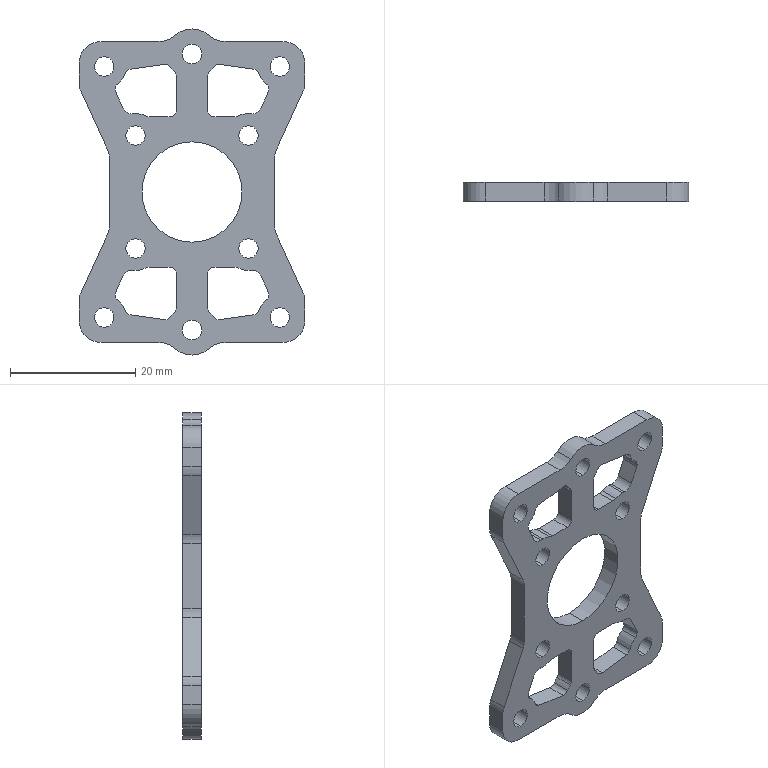Part | SolidWorks | features Fillet 3, Extrusion 1, ICE 1 | 1 solid | 119 faces | box 36 x 3 x 52 mm | volume 2909 mm3 | cylinder 87 | plane 32 | commonest cylinder face diameters 7 x26 2 x22 3.1 x20 3 x10 8 x7 16 x2